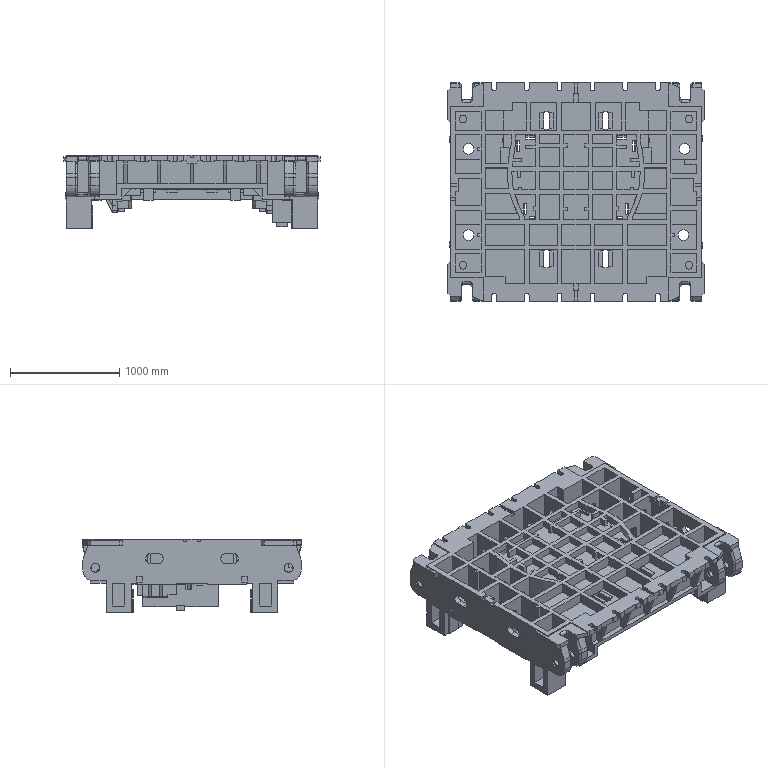Part | NX | features solid 2 | 1 solid | 1971 faces | box 2350 x 2010 x 670 mm | volume 672928428 mm3 | plane 1668 | cylinder 247 | spline 28 | torus 28 | commonest cylinder face diameters 80 x56 83 x48 40 x40 20 x16 60 x16 79 x16